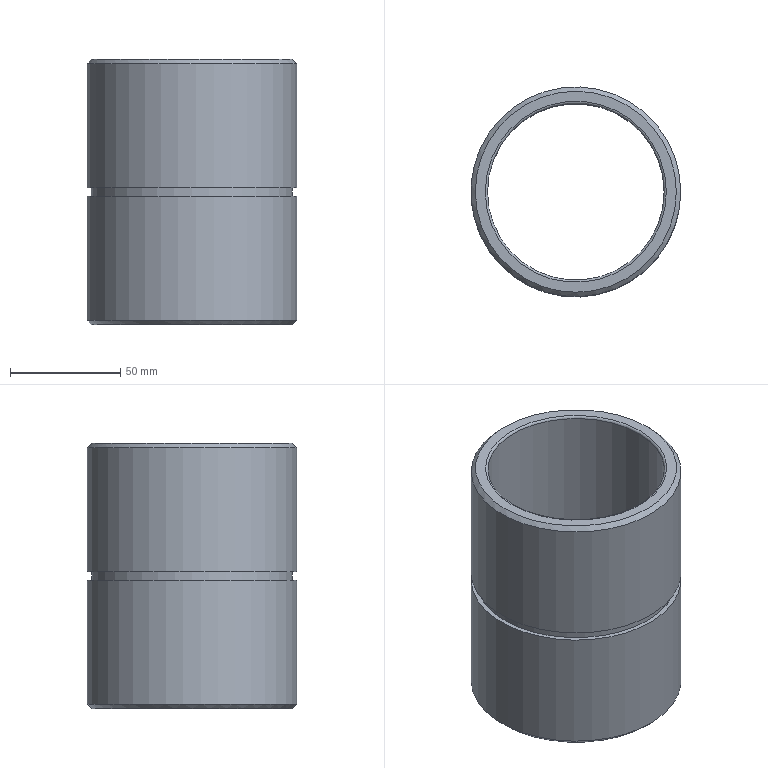Part | STEP file | solid 211 | 1 solid | 12 faces | box 95 x 95 x 120 mm | volume 243778 mm3 | plane 4 | cylinder 4 | torus 2 | cone 2 | commonest cylinder face diameters 95 x2 80 x1 91 x1